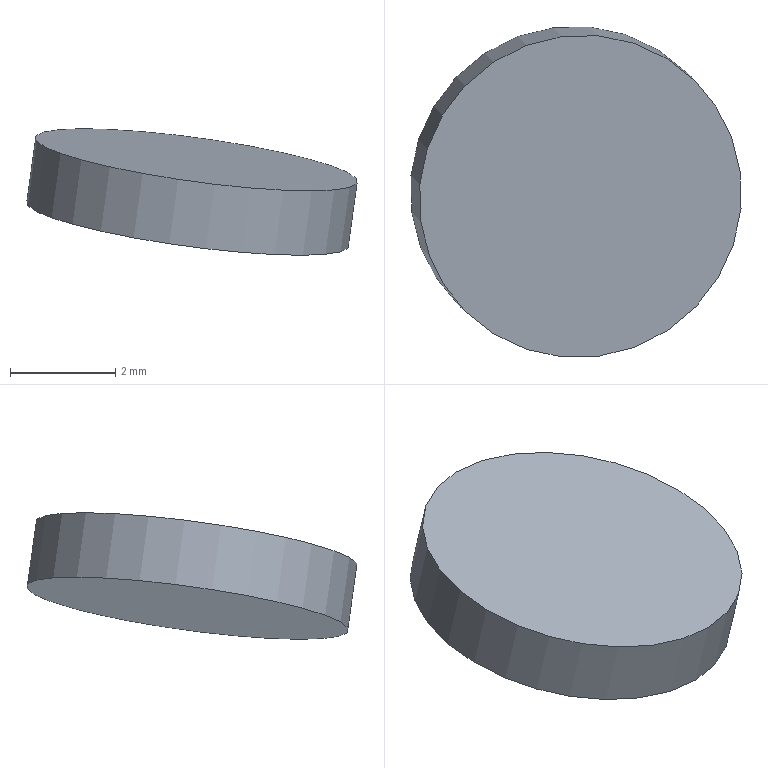Part | STEP file | gslz 2016.10.28-13_id1086_x_t | 1 solid | 3 faces | box 6.311 x 6.312 x 2.41 mm | volume 37.737 mm3 | spline 2 | cylinder 1 | commonest cylinder face diameters 6.2 x1
STEP:
#1=CARTESIAN_POINT('',(0.,0.,0.));
#2=DIRECTION('',(0.,0.,1.));
#3=DIRECTION('',(1.,0.,0.));
#4=AXIS2_PLACEMENT_3D('',#1,#2,#3);
#5=CARTESIAN_POINT('',(775.863,213.366,0.09839));
#6=VERTEX_POINT('',#5);
#7=CARTESIAN_POINT('',(771.479,208.982,0.09841));
#8=VERTEX_POINT('',#7);
#9=CARTESIAN_POINT('',(775.863,213.366,0.09839));
#10=CARTESIAN_POINT('',(775.855,213.374,0.1005));
#11=CARTESIAN_POINT('',(775.848,213.381,0.1026));
#12=CARTESIAN_POINT('',(775.84,213.389,0.1048));
#13=CARTESIAN_POINT('',(775.596,213.627,0.171));
#14=CARTESIAN_POINT('',(775.308,213.826,0.238));
#15=CARTESIAN_POINT('',(774.998,213.969,0.3002));
#16=CARTESIAN_POINT('',(774.688,214.111,0.3624));
#17=CARTESIAN_POINT('',(774.348,214.202,0.4216));
#18=CARTESIAN_POINT('',(774.006,214.233,0.4729));
#19=CARTESIAN_POINT('',(773.664,214.264,0.5241));
#20=CARTESIAN_POINT('',(773.311,214.237,0.5688));
#21=CARTESIAN_POINT('',(772.976,214.153,0.6033));
#22=CARTESIAN_POINT('',(772.641,214.069,0.6378));
#23=CARTESIAN_POINT('',(772.315,213.926,0.663));
#24=CARTESIAN_POINT('',(772.025,213.736,0.6768));
#25=CARTESIAN_POINT('',(771.843,213.618,0.6855));
#26=CARTESIAN_POINT('',(771.673,213.479,0.6899));
#27=CARTESIAN_POINT('',(771.519,213.326,0.6899));
#28=CARTESIAN_POINT('',(771.274,213.08,0.6899));
#29=CARTESIAN_POINT('',(771.067,212.79,0.6785));
#30=CARTESIAN_POINT('',(770.915,212.479,0.6566));
#31=CARTESIAN_POINT('',(770.763,212.168,0.6347));
#32=CARTESIAN_POINT('',(770.663,211.827,0.6017));
#33=CARTESIAN_POINT('',(770.622,211.485,0.5603));
#34=CARTESIAN_POINT('',(770.58,211.143,0.5189));
#35=CARTESIAN_POINT('',(770.598,210.79,0.4681));
#36=CARTESIAN_POINT('',(770.672,210.456,0.412));
#37=CARTESIAN_POINT('',(770.746,210.122,0.3558));
#38=CARTESIAN_POINT('',(770.879,209.797,0.2928));
#39=CARTESIAN_POINT('',(771.06,209.508,0.2283));
#40=CARTESIAN_POINT('',(771.179,209.318,0.1858));
#41=CARTESIAN_POINT('',(771.321,209.14,0.142));
#42=CARTESIAN_POINT('',(771.479,208.982,0.09841));
#43=B_SPLINE_CURVE_WITH_KNOTS('',3,(#9,#10,#11,#12,#13,#14,#15,#16,#17,#18,#19,#20,#21,#22,#23,#24,#25,#26,#27,#28,#29,#30,#31,#32,#33,#34,#35,#36,#37,#38,#39,#40,#41,#42),.UNSPECIFIED.,.F.,.F.,(4,3,3,3,3,3,3,3,3,3,3,4),(0.,0.003402,0.1108,0.2183,0.3257,0.4331,0.4998,0.6072,0.7146,0.822,0.9295,1.),.UNSPECIFIED.);
#44=CARTESIAN_POINT('',(773.503,211.343,-1.129));
#45=DIRECTION('',(0.1349,-0.1349,0.9816));
#46=DIRECTION('',(-0.01175,-0.9908,-0.1346));
#47=AXIS2_PLACEMENT_3D('',#44,#45,#46);
#48=CYLINDRICAL_SURFACE('',#47,3.1);
#49=CARTESIAN_POINT('',(8.642,1.25));
#50=CARTESIAN_POINT('',(11.784,1.25));
#51=B_SPLINE_CURVE_WITH_KNOTS('',1,(#49,#50),.UNSPECIFIED.,.F.,.F.,(2,2),(0.,1.),.PIECEWISE_BEZIER_KNOTS.);
#52=(GEOMETRIC_REPRESENTATION_CONTEXT(2)PARAMETRIC_REPRESENTATION_CONTEXT()REPRESENTATION_CONTEXT('',''));
#53=DEFINITIONAL_REPRESENTATION('',(#51),#52);
#54=PCURVE('',#48,#53);
#55=CARTESIAN_POINT('',(582.842,140.622,16.631));
#56=CARTESIAN_POINT('',(603.987,119.477,10.818));
#57=CARTESIAN_POINT('',(625.133,98.331,5.005));
#58=CARTESIAN_POINT('',(646.279,77.185,-0.8076));
#59=CARTESIAN_POINT('',(667.424,56.039,-6.62));
#60=CARTESIAN_POINT('',(688.57,34.894,-12.433));
#61=CARTESIAN_POINT('',(618.357,176.138,16.631));
#62=CARTESIAN_POINT('',(639.503,154.992,10.818));
#63=CARTESIAN_POINT('',(660.649,133.847,5.005));
#64=CARTESIAN_POINT('',(681.795,112.701,-0.8078));
#65=CARTESIAN_POINT('',(702.94,91.555,-6.621));
#66=CARTESIAN_POINT('',(724.086,70.41,-12.434));
#67=CARTESIAN_POINT('',(653.873,211.654,16.631));
#68=CARTESIAN_POINT('',(675.019,190.508,10.818));
#69=CARTESIAN_POINT('',(696.165,169.363,5.005));
#70=CARTESIAN_POINT('',(717.31,148.217,-0.808));
#71=CARTESIAN_POINT('',(738.456,127.071,-6.621));
#72=CARTESIAN_POINT('',(759.602,105.925,-12.434));
#73=CARTESIAN_POINT('',(689.389,247.17,16.63));
#74=CARTESIAN_POINT('',(710.535,226.024,10.818));
#75=CARTESIAN_POINT('',(731.68,204.878,5.005));
#76=CARTESIAN_POINT('',(752.826,183.733,-0.8082));
#77=CARTESIAN_POINT('',(773.972,162.587,-6.621));
#78=CARTESIAN_POINT('',(795.118,141.441,-12.434));
#79=CARTESIAN_POINT('',(724.905,282.686,16.63));
#80=CARTESIAN_POINT('',(746.051,261.54,10.817));
#81=CARTESIAN_POINT('',(767.196,240.394,5.005));
#82=CARTESIAN_POINT('',(788.342,219.248,-0.8083));
#83=CARTESIAN_POINT('',(809.488,198.103,-6.621));
#84=CARTESIAN_POINT('',(830.633,176.957,-12.434));
#85=CARTESIAN_POINT('',(760.421,318.201,16.63));
#86=CARTESIAN_POINT('',(781.566,297.056,10.817));
#87=CARTESIAN_POINT('',(802.712,275.91,5.004));
#88=CARTESIAN_POINT('',(823.858,254.764,-0.8085));
#89=CARTESIAN_POINT('',(845.003,233.618,-6.621));
#90=CARTESIAN_POINT('',(866.149,212.473,-12.434));
#91=B_SPLINE_SURFACE_WITH_KNOTS('',5,5,((#55,#56,#57,#58,#59,#60),(#61,#62,#63,#64,#65,#66),(#67,#68,#69,#70,#71,#72),(#73,#74,#75,#76,#77,#78),(#79,#80,#81,#82,#83,#84),(#85,#86,#87,#88,#89,#90)),.UNSPECIFIED.,.F.,.F.,.F.,(6,6),(6,6),(0.,1.),(0.,1.),.PIECEWISE_BEZIER_KNOTS.);
#92=CARTESIAN_POINT('',(0.7483,0.5688));
#93=CARTESIAN_POINT('',(0.7483,0.5683));
#94=CARTESIAN_POINT('',(0.7483,0.5674));
#95=CARTESIAN_POINT('',(0.7482,0.5659));
#96=CARTESIAN_POINT('',(0.748,0.5645));
#97=CARTESIAN_POINT('',(0.7478,0.5631));
#98=CARTESIAN_POINT('',(0.7475,0.5617));
#99=CARTESIAN_POINT('',(0.7472,0.5603));
#100=CARTESIAN_POINT('',(0.7468,0.559));
#101=CARTESIAN_POINT('',(0.7463,0.5578));
#102=CARTESIAN_POINT('',(0.7458,0.5566));
#103=CARTESIAN_POINT('',(0.7453,0.5555));
#104=CARTESIAN_POINT('',(0.7447,0.5544));
#105=CARTESIAN_POINT('',(0.744,0.5534));
#106=CARTESIAN_POINT('',(0.7434,0.5525));
#107=CARTESIAN_POINT('',(0.7426,0.5517));
#108=CARTESIAN_POINT('',(0.7419,0.5509));
#109=CARTESIAN_POINT('',(0.7411,0.5503));
#110=CARTESIAN_POINT('',(0.7403,0.5497));
#111=CARTESIAN_POINT('',(0.7394,0.5493));
#112=CARTESIAN_POINT('',(0.7386,0.5489));
#113=CARTESIAN_POINT('',(0.7377,0.5486));
#114=CARTESIAN_POINT('',(0.7368,0.5485));
#115=CARTESIAN_POINT('',(0.7359,0.5484));
#116=CARTESIAN_POINT('',(0.7351,0.5485));
#117=CARTESIAN_POINT('',(0.7342,0.5486));
#118=CARTESIAN_POINT('',(0.7333,0.5489));
#119=CARTESIAN_POINT('',(0.7325,0.5493));
#120=CARTESIAN_POINT('',(0.7316,0.5497));
#121=CARTESIAN_POINT('',(0.7308,0.5503));
#122=CARTESIAN_POINT('',(0.73,0.5509));
#123=CARTESIAN_POINT('',(0.7293,0.5517));
#124=CARTESIAN_POINT('',(0.7285,0.5525));
#125=CARTESIAN_POINT('',(0.7279,0.5534));
#126=CARTESIAN_POINT('',(0.7272,0.5544));
#127=CARTESIAN_POINT('',(0.7266,0.5555));
#128=CARTESIAN_POINT('',(0.7261,0.5566));
#129=CARTESIAN_POINT('',(0.7256,0.5578));
#130=CARTESIAN_POINT('',(0.7251,0.559));
#131=CARTESIAN_POINT('',(0.7247,0.5603));
#132=CARTESIAN_POINT('',(0.7244,0.5617));
#133=CARTESIAN_POINT('',(0.7241,0.5631));
#134=CARTESIAN_POINT('',(0.7239,0.5645));
#135=CARTESIAN_POINT('',(0.7237,0.5659));
#136=CARTESIAN_POINT('',(0.7236,0.5674));
#137=CARTESIAN_POINT('',(0.7236,0.5683));
#138=CARTESIAN_POINT('',(0.7236,0.5688));
#139=B_SPLINE_CURVE_WITH_KNOTS('',3,(#92,#93,#94,#95,#96,#97,#98,#99,#100,#101,#102,#103,#104,#105,#106,#107,#108,#109,#110,#111,#112,#113,#114,#115,#116,#117,#118,#119,#120,#121,#122,#123,#124,#125,#126,#127,#128,#129,#130,#131,#132,#133,#134,#135,#136,#137,#138),.UNSPECIFIED.,.F.,.F.,(4,1,1,1,1,1,1,1,1,1,1,1,1,1,1,1,1,1,1,1,1,1,1,1,1,1,1,1,1,1,1,1,1,1,1,1,1,1,1,1,1,1,1,1,4),(0.,0.02273,0.04545,0.06818,0.09091,0.1136,0.1364,0.1591,0.1818,0.2045,0.2273,0.25,0.2727,0.2955,0.3182,0.3409,0.3636,0.3864,0.4091,0.4318,0.4545,0.4773,0.5,0.5227,0.5455,0.5682,0.5909,0.6136,0.6364,0.6591,0.6818,0.7045,0.7273,0.75,0.7727,0.7955,0.8182,0.8409,0.8636,0.8864,0.9091,0.9318,0.9545,0.9773,1.),.QUASI_UNIFORM_KNOTS.);
#140=(GEOMETRIC_REPRESENTATION_CONTEXT(2)PARAMETRIC_REPRESENTATION_CONTEXT()REPRESENTATION_CONTEXT('',''));
#141=DEFINITIONAL_REPRESENTATION('',(#139),#140);
#142=PCURVE('',#91,#141);
#143=SURFACE_CURVE('',#43,(#54,#142),.PCURVE_S1.);
#144=EDGE_CURVE('',#6,#8,#143,.T.);
#145=ORIENTED_EDGE('',*,*,#144,.F.);
#146=CARTESIAN_POINT('',(771.479,208.982,0.09841));
#147=CARTESIAN_POINT('',(771.487,208.974,0.09629));
#148=CARTESIAN_POINT('',(771.495,208.967,0.09416));
#149=CARTESIAN_POINT('',(771.502,208.959,0.09204));
#150=CARTESIAN_POINT('',(771.746,208.721,0.02584));
#151=CARTESIAN_POINT('',(772.035,208.522,-0.04115));
#152=CARTESIAN_POINT('',(772.345,208.379,-0.1034));
#153=CARTESIAN_POINT('',(772.655,208.237,-0.1656));
#154=CARTESIAN_POINT('',(772.995,208.146,-0.2248));
#155=CARTESIAN_POINT('',(773.337,208.115,-0.2761));
#156=CARTESIAN_POINT('',(773.678,208.084,-0.3273));
#157=CARTESIAN_POINT('',(774.031,208.111,-0.372));
#158=CARTESIAN_POINT('',(774.366,208.195,-0.4065));
#159=CARTESIAN_POINT('',(774.701,208.279,-0.441));
#160=CARTESIAN_POINT('',(775.027,208.422,-0.4662));
#161=CARTESIAN_POINT('',(775.317,208.612,-0.48));
#162=CARTESIAN_POINT('',(775.499,208.73,-0.4887));
#163=CARTESIAN_POINT('',(775.669,208.869,-0.4931));
#164=CARTESIAN_POINT('',(775.823,209.022,-0.4931));
#165=CARTESIAN_POINT('',(776.068,209.268,-0.4931));
#166=CARTESIAN_POINT('',(776.275,209.558,-0.4817));
#167=CARTESIAN_POINT('',(776.427,209.869,-0.4598));
#168=CARTESIAN_POINT('',(776.579,210.18,-0.4379));
#169=CARTESIAN_POINT('',(776.68,210.521,-0.4049));
#170=CARTESIAN_POINT('',(776.721,210.863,-0.3635));
#171=CARTESIAN_POINT('',(776.762,211.205,-0.3221));
#172=CARTESIAN_POINT('',(776.745,211.558,-0.2713));
#173=CARTESIAN_POINT('',(776.67,211.892,-0.2152));
#174=CARTESIAN_POINT('',(776.596,212.226,-0.159));
#175=CARTESIAN_POINT('',(776.463,212.551,-0.09604));
#176=CARTESIAN_POINT('',(776.282,212.84,-0.03145));
#177=CARTESIAN_POINT('',(776.163,213.03,0.01103));
#178=CARTESIAN_POINT('',(776.022,213.208,0.05484));
#179=CARTESIAN_POINT('',(775.863,213.366,0.09839));
#180=B_SPLINE_CURVE_WITH_KNOTS('',3,(#146,#147,#148,#149,#150,#151,#152,#153,#154,#155,#156,#157,#158,#159,#160,#161,#162,#163,#164,#165,#166,#167,#168,#169,#170,#171,#172,#173,#174,#175,#176,#177,#178,#179),.UNSPECIFIED.,.F.,.F.,(4,3,3,3,3,3,3,3,3,3,3,4),(0.,0.003402,0.1108,0.2183,0.3257,0.4331,0.4998,0.6072,0.7146,0.822,0.9295,1.),.UNSPECIFIED.);
#181=CARTESIAN_POINT('',(5.5,1.25));
#182=CARTESIAN_POINT('',(8.642,1.25));
#183=B_SPLINE_CURVE_WITH_KNOTS('',1,(#181,#182),.UNSPECIFIED.,.F.,.F.,(2,2),(0.,1.),.PIECEWISE_BEZIER_KNOTS.);
#184=(GEOMETRIC_REPRESENTATION_CONTEXT(2)PARAMETRIC_REPRESENTATION_CONTEXT()REPRESENTATION_CONTEXT('',''));
#185=DEFINITIONAL_REPRESENTATION('',(#183),#184);
#186=PCURVE('',#48,#185);
#187=CARTESIAN_POINT('',(0.7236,0.5688));
#188=CARTESIAN_POINT('',(0.7236,0.5693));
#189=CARTESIAN_POINT('',(0.7236,0.5703));
#190=CARTESIAN_POINT('',(0.7237,0.5717));
#191=CARTESIAN_POINT('',(0.7239,0.5731));
#192=CARTESIAN_POINT('',(0.7241,0.5745));
#193=CARTESIAN_POINT('',(0.7244,0.5759));
#194=CARTESIAN_POINT('',(0.7247,0.5773));
#195=CARTESIAN_POINT('',(0.7251,0.5786));
#196=CARTESIAN_POINT('',(0.7256,0.5798));
#197=CARTESIAN_POINT('',(0.7261,0.581));
#198=CARTESIAN_POINT('',(0.7266,0.5821));
#199=CARTESIAN_POINT('',(0.7272,0.5832));
#200=CARTESIAN_POINT('',(0.7279,0.5842));
#201=CARTESIAN_POINT('',(0.7286,0.5851));
#202=CARTESIAN_POINT('',(0.7293,0.5859));
#203=CARTESIAN_POINT('',(0.73,0.5867));
#204=CARTESIAN_POINT('',(0.7308,0.5873));
#205=CARTESIAN_POINT('',(0.7316,0.5879));
#206=CARTESIAN_POINT('',(0.7325,0.5883));
#207=CARTESIAN_POINT('',(0.7333,0.5887));
#208=CARTESIAN_POINT('',(0.7342,0.589));
#209=CARTESIAN_POINT('',(0.7351,0.5891));
#210=CARTESIAN_POINT('',(0.736,0.5892));
#211=CARTESIAN_POINT('',(0.7368,0.5891));
#212=CARTESIAN_POINT('',(0.7377,0.589));
#213=CARTESIAN_POINT('',(0.7386,0.5887));
#214=CARTESIAN_POINT('',(0.7394,0.5883));
#215=CARTESIAN_POINT('',(0.7403,0.5879));
#216=CARTESIAN_POINT('',(0.7411,0.5873));
#217=CARTESIAN_POINT('',(0.7419,0.5867));
#218=CARTESIAN_POINT('',(0.7426,0.5859));
#219=CARTESIAN_POINT('',(0.7434,0.5851));
#220=CARTESIAN_POINT('',(0.7441,0.5842));
#221=CARTESIAN_POINT('',(0.7447,0.5832));
#222=CARTESIAN_POINT('',(0.7453,0.5821));
#223=CARTESIAN_POINT('',(0.7459,0.581));
#224=CARTESIAN_POINT('',(0.7464,0.5798));
#225=CARTESIAN_POINT('',(0.7468,0.5786));
#226=CARTESIAN_POINT('',(0.7472,0.5773));
#227=CARTESIAN_POINT('',(0.7475,0.5759));
#228=CARTESIAN_POINT('',(0.7478,0.5745));
#229=CARTESIAN_POINT('',(0.748,0.5731));
#230=CARTESIAN_POINT('',(0.7482,0.5717));
#231=CARTESIAN_POINT('',(0.7483,0.5703));
#232=CARTESIAN_POINT('',(0.7483,0.5693));
#233=CARTESIAN_POINT('',(0.7483,0.5688));
#234=B_SPLINE_CURVE_WITH_KNOTS('',3,(#187,#188,#189,#190,#191,#192,#193,#194,#195,#196,#197,#198,#199,#200,#201,#202,#203,#204,#205,#206,#207,#208,#209,#210,#211,#212,#213,#214,#215,#216,#217,#218,#219,#220,#221,#222,#223,#224,#225,#226,#227,#228,#229,#230,#231,#232,#233),.UNSPECIFIED.,.F.,.F.,(4,1,1,1,1,1,1,1,1,1,1,1,1,1,1,1,1,1,1,1,1,1,1,1,1,1,1,1,1,1,1,1,1,1,1,1,1,1,1,1,1,1,1,1,4),(0.,0.02273,0.04545,0.06818,0.09091,0.1136,0.1364,0.1591,0.1818,0.2045,0.2273,0.25,0.2727,0.2955,0.3182,0.3409,0.3636,0.3864,0.4091,0.4318,0.4545,0.4773,0.5,0.5227,0.5455,0.5682,0.5909,0.6136,0.6364,0.6591,0.6818,0.7045,0.7273,0.75,0.7727,0.7955,0.8182,0.8409,0.8636,0.8864,0.9091,0.9318,0.9545,0.9773,1.),.QUASI_UNIFORM_KNOTS.);
#235=(GEOMETRIC_REPRESENTATION_CONTEXT(2)PARAMETRIC_REPRESENTATION_CONTEXT()REPRESENTATION_CONTEXT('',''));
#236=DEFINITIONAL_REPRESENTATION('',(#234),#235);
#237=PCURVE('',#91,#236);
#238=SURFACE_CURVE('',#180,(#186,#237),.PCURVE_S1.);
#239=EDGE_CURVE('',#8,#6,#238,.T.);
#240=ORIENTED_EDGE('',*,*,#239,.F.);
#241=CARTESIAN_POINT('',(771.31,209.151,-1.129));
#242=VERTEX_POINT('',#241);
#243=CARTESIAN_POINT('',(771.31,209.151,-1.129));
#244=CARTESIAN_POINT('',(771.479,208.982,0.09841));
#245=B_SPLINE_CURVE_WITH_KNOTS('',1,(#243,#244),.UNSPECIFIED.,.F.,.F.,(2,2),(0.,1.25),.PIECEWISE_BEZIER_KNOTS.);
#246=CARTESIAN_POINT('',(5.5,0.));
#247=DIRECTION('',(0.,1.));
#248=VECTOR('',#247,1.);
#249=LINE('',#246,#248);
#250=(GEOMETRIC_REPRESENTATION_CONTEXT(2)PARAMETRIC_REPRESENTATION_CONTEXT()REPRESENTATION_CONTEXT('',''));
#251=DEFINITIONAL_REPRESENTATION('',(#249),#250);
#252=PCURVE('',#48,#251);
#253=CARTESIAN_POINT('',(11.784,0.));
#254=DIRECTION('',(0.,1.));
#255=VECTOR('',#254,1.);
#256=LINE('',#253,#255);
#257=(GEOMETRIC_REPRESENTATION_CONTEXT(2)PARAMETRIC_REPRESENTATION_CONTEXT()REPRESENTATION_CONTEXT('',''));
#258=DEFINITIONAL_REPRESENTATION('',(#256),#257);
#259=PCURVE('',#48,#258);
#260=SEAM_CURVE('',#245,(#252,#259),.PCURVE_S1.);
#261=EDGE_CURVE('',#242,#8,#260,.T.);
#262=ORIENTED_EDGE('',*,*,#261,.F.);
#263=CARTESIAN_POINT('',(775.695,213.535,-1.129));
#264=VERTEX_POINT('',#263);
#265=CARTESIAN_POINT('',(771.31,209.151,-1.129));
#266=CARTESIAN_POINT('',(771.318,209.143,-1.131));
#267=CARTESIAN_POINT('',(771.326,209.135,-1.133));
#268=CARTESIAN_POINT('',(771.334,209.128,-1.135));
#269=CARTESIAN_POINT('',(771.577,208.889,-1.201));
#270=CARTESIAN_POINT('',(771.866,208.691,-1.268));
#271=CARTESIAN_POINT('',(772.176,208.548,-1.33));
#272=CARTESIAN_POINT('',(772.486,208.405,-1.393));
#273=CARTESIAN_POINT('',(772.826,208.315,-1.452));
#274=CARTESIAN_POINT('',(773.168,208.284,-1.503));
#275=CARTESIAN_POINT('',(773.51,208.253,-1.554));
#276=CARTESIAN_POINT('',(773.863,208.28,-1.599));
#277=CARTESIAN_POINT('',(774.197,208.364,-1.634));
#278=CARTESIAN_POINT('',(774.532,208.448,-1.668));
#279=CARTESIAN_POINT('',(774.858,208.591,-1.693));
#280=CARTESIAN_POINT('',(775.149,208.78,-1.707));
#281=CARTESIAN_POINT('',(775.33,208.899,-1.716));
#282=CARTESIAN_POINT('',(775.501,209.037,-1.72));
#283=CARTESIAN_POINT('',(775.654,209.191,-1.72));
#284=CARTESIAN_POINT('',(775.9,209.436,-1.72));
#285=CARTESIAN_POINT('',(776.107,209.727,-1.709));
#286=CARTESIAN_POINT('',(776.259,210.038,-1.687));
#287=CARTESIAN_POINT('',(776.41,210.349,-1.665));
#288=CARTESIAN_POINT('',(776.511,210.69,-1.632));
#289=CARTESIAN_POINT('',(776.552,211.032,-1.591));
#290=CARTESIAN_POINT('',(776.593,211.374,-1.549));
#291=CARTESIAN_POINT('',(776.576,211.727,-1.498));
#292=CARTESIAN_POINT('',(776.502,212.061,-1.442));
#293=CARTESIAN_POINT('',(776.428,212.395,-1.386));
#294=CARTESIAN_POINT('',(776.295,212.72,-1.323));
#295=CARTESIAN_POINT('',(776.113,213.009,-1.258));
#296=CARTESIAN_POINT('',(775.994,213.199,-1.216));
#297=CARTESIAN_POINT('',(775.853,213.376,-1.172));
#298=CARTESIAN_POINT('',(775.695,213.535,-1.129));
#299=B_SPLINE_CURVE_WITH_KNOTS('',3,(#265,#266,#267,#268,#269,#270,#271,#272,#273,#274,#275,#276,#277,#278,#279,#280,#281,#282,#283,#284,#285,#286,#287,#288,#289,#290,#291,#292,#293,#294,#295,#296,#297,#298),.UNSPECIFIED.,.F.,.F.,(4,3,3,3,3,3,3,3,3,3,3,4),(0.,0.003402,0.1108,0.2183,0.3257,0.4331,0.4998,0.6072,0.7146,0.822,0.9295,1.),.UNSPECIFIED.);
#300=CARTESIAN_POINT('',(5.5,0.));
#301=CARTESIAN_POINT('',(8.642,0.));
#302=B_SPLINE_CURVE_WITH_KNOTS('',1,(#300,#301),.UNSPECIFIED.,.F.,.F.,(2,2),(0.,1.),.PIECEWISE_BEZIER_KNOTS.);
#303=(GEOMETRIC_REPRESENTATION_CONTEXT(2)PARAMETRIC_REPRESENTATION_CONTEXT()REPRESENTATION_CONTEXT('',''));
#304=DEFINITIONAL_REPRESENTATION('',(#302),#303);
#305=PCURVE('',#48,#304);
#306=CARTESIAN_POINT('',(769.107,211.302,-0.53));
#307=CARTESIAN_POINT('',(770.558,209.85,-0.9291));
#308=CARTESIAN_POINT('',(772.01,208.399,-1.328));
#309=CARTESIAN_POINT('',(773.462,206.947,-1.727));
#310=CARTESIAN_POINT('',(770.585,212.781,-0.53));
#311=CARTESIAN_POINT('',(772.037,211.329,-0.9291));
#312=CARTESIAN_POINT('',(773.489,209.877,-1.328));
#313=CARTESIAN_POINT('',(774.941,208.426,-1.727));
#314=CARTESIAN_POINT('',(772.064,214.26,-0.53));
#315=CARTESIAN_POINT('',(773.516,212.808,-0.9291));
#316=CARTESIAN_POINT('',(774.968,211.356,-1.328));
#317=CARTESIAN_POINT('',(776.42,209.905,-1.727));
#318=CARTESIAN_POINT('',(773.543,215.739,-0.53));
#319=CARTESIAN_POINT('',(774.995,214.287,-0.9291));
#320=CARTESIAN_POINT('',(776.447,212.835,-1.328));
#321=CARTESIAN_POINT('',(777.898,211.383,-1.727));
#322=B_SPLINE_SURFACE_WITH_KNOTS('',3,3,((#306,#307,#308,#309),(#310,#311,#312,#313),(#314,#315,#316,#317),(#318,#319,#320,#321)),.UNSPECIFIED.,.F.,.F.,.F.,(4,4),(4,4),(0.,1.),(0.,1.),.PIECEWISE_BEZIER_KNOTS.);
#323=CARTESIAN_POINT('',(0.005929,0.5));
#324=CARTESIAN_POINT('',(0.005927,0.5117));
#325=CARTESIAN_POINT('',(0.006781,0.5352));
#326=CARTESIAN_POINT('',(0.01059,0.5703));
#327=CARTESIAN_POINT('',(0.01687,0.6052));
#328=CARTESIAN_POINT('',(0.02559,0.6394));
#329=CARTESIAN_POINT('',(0.03666,0.6728));
#330=CARTESIAN_POINT('',(0.05017,0.7053));
#331=CARTESIAN_POINT('',(0.06601,0.7369));
#332=CARTESIAN_POINT('',(0.08405,0.7673));
#333=CARTESIAN_POINT('',(0.1042,0.7964));
#334=CARTESIAN_POINT('',(0.1262,0.8237));
#335=CARTESIAN_POINT('',(0.1502,0.8495));
#336=CARTESIAN_POINT('',(0.1761,0.8736));
#337=CARTESIAN_POINT('',(0.2037,0.8958));
#338=CARTESIAN_POINT('',(0.2326,0.916));
#339=CARTESIAN_POINT('',(0.2628,0.9339));
#340=CARTESIAN_POINT('',(0.2944,0.9497));
#341=CARTESIAN_POINT('',(0.3271,0.9632));
#342=CARTESIAN_POINT('',(0.3606,0.9744));
#343=CARTESIAN_POINT('',(0.3946,0.9831));
#344=CARTESIAN_POINT('',(0.4296,0.9895));
#345=CARTESIAN_POINT('',(0.4649,0.9932));
#346=CARTESIAN_POINT('',(0.5005,0.9945));
#347=CARTESIAN_POINT('',(0.5355,0.9932));
#348=CARTESIAN_POINT('',(0.5707,0.9894));
#349=CARTESIAN_POINT('',(0.6055,0.9831));
#350=CARTESIAN_POINT('',(0.6397,0.9743));
#351=CARTESIAN_POINT('',(0.673,0.9632));
#352=CARTESIAN_POINT('',(0.7056,0.9497));
#353=CARTESIAN_POINT('',(0.7372,0.9338));
#354=CARTESIAN_POINT('',(0.7676,0.9158));
#355=CARTESIAN_POINT('',(0.7966,0.8956));
#356=CARTESIAN_POINT('',(0.8239,0.8736));
#357=CARTESIAN_POINT('',(0.8498,0.8495));
#358=CARTESIAN_POINT('',(0.8738,0.8236));
#359=CARTESIAN_POINT('',(0.896,0.7961));
#360=CARTESIAN_POINT('',(0.9161,0.7671));
#361=CARTESIAN_POINT('',(0.934,0.7369));
#362=CARTESIAN_POINT('',(0.9498,0.7053));
#363=CARTESIAN_POINT('',(0.9633,0.6726));
#364=CARTESIAN_POINT('',(0.9745,0.639));
#365=CARTESIAN_POINT('',(0.9832,0.605));
#366=CARTESIAN_POINT('',(0.9895,0.5703));
#367=CARTESIAN_POINT('',(0.9932,0.5352));
#368=CARTESIAN_POINT('',(0.9941,0.5117));
#369=CARTESIAN_POINT('',(0.9941,0.5));
#370=B_SPLINE_CURVE_WITH_KNOTS('',3,(#323,#324,#325,#326,#327,#328,#329,#330,#331,#332,#333,#334,#335,#336,#337,#338,#339,#340,#341,#342,#343,#344,#345,#346,#347,#348,#349,#350,#351,#352,#353,#354,#355,#356,#357,#358,#359,#360,#361,#362,#363,#364,#365,#366,#367,#368,#369),.UNSPECIFIED.,.F.,.F.,(4,1,1,1,1,1,1,1,1,1,1,1,1,1,1,1,1,1,1,1,1,1,1,1,1,1,1,1,1,1,1,1,1,1,1,1,1,1,1,1,1,1,1,1,4),(0.,0.02273,0.04545,0.06818,0.09091,0.1136,0.1364,0.1591,0.1818,0.2045,0.2273,0.25,0.2727,0.2955,0.3182,0.3409,0.3636,0.3864,0.4091,0.4318,0.4545,0.4773,0.5,0.5227,0.5455,0.5682,0.5909,0.6136,0.6364,0.6591,0.6818,0.7045,0.7273,0.75,0.7727,0.7955,0.8182,0.8409,0.8636,0.8864,0.9091,0.9318,0.9545,0.9773,1.),.QUASI_UNIFORM_KNOTS.);
#371=(GEOMETRIC_REPRESENTATION_CONTEXT(2)PARAMETRIC_REPRESENTATION_CONTEXT()REPRESENTATION_CONTEXT('',''));
#372=DEFINITIONAL_REPRESENTATION('',(#370),#371);
#373=PCURVE('',#322,#372);
#374=SURFACE_CURVE('',#299,(#305,#373),.PCURVE_S1.);
#375=EDGE_CURVE('',#242,#264,#374,.T.);
#376=ORIENTED_EDGE('',*,*,#375,.T.);
#377=CARTESIAN_POINT('',(775.695,213.535,-1.129));
#378=CARTESIAN_POINT('',(775.687,213.542,-1.127));
#379=CARTESIAN_POINT('',(775.679,213.55,-1.124));
#380=CARTESIAN_POINT('',(775.671,213.558,-1.122));
#381=CARTESIAN_POINT('',(775.428,213.796,-1.056));
#382=CARTESIAN_POINT('',(775.139,213.995,-0.9891));
#383=CARTESIAN_POINT('',(774.829,214.137,-0.9268));
#384=CARTESIAN_POINT('',(774.519,214.28,-0.8646));
#385=CARTESIAN_POINT('',(774.179,214.371,-0.8054));
#386=CARTESIAN_POINT('',(773.837,214.402,-0.7542));
#387=CARTESIAN_POINT('',(773.495,214.433,-0.7029));
#388=CARTESIAN_POINT('',(773.142,214.405,-0.6582));
#389=CARTESIAN_POINT('',(772.808,214.321,-0.6237));
#390=CARTESIAN_POINT('',(772.473,214.237,-0.5892));
#391=CARTESIAN_POINT('',(772.147,214.095,-0.564));
#392=CARTESIAN_POINT('',(771.856,213.905,-0.5502));
#393=CARTESIAN_POINT('',(771.675,213.786,-0.5415));
#394=CARTESIAN_POINT('',(771.504,213.648,-0.5371));
#395=CARTESIAN_POINT('',(771.351,213.494,-0.5371));
#396=CARTESIAN_POINT('',(771.105,213.249,-0.5371));
#397=CARTESIAN_POINT('',(770.898,212.959,-0.5486));
#398=CARTESIAN_POINT('',(770.746,212.648,-0.5705));
#399=CARTESIAN_POINT('',(770.595,212.336,-0.5924));
#400=CARTESIAN_POINT('',(770.494,211.996,-0.6254));
#401=CARTESIAN_POINT('',(770.453,211.654,-0.6667));
#402=CARTESIAN_POINT('',(770.412,211.312,-0.7081));
#403=CARTESIAN_POINT('',(770.429,210.959,-0.7589));
#404=CARTESIAN_POINT('',(770.503,210.625,-0.8151));
#405=CARTESIAN_POINT('',(770.577,210.29,-0.8712));
#406=CARTESIAN_POINT('',(770.71,209.965,-0.9342));
#407=CARTESIAN_POINT('',(770.892,209.676,-0.9988));
#408=CARTESIAN_POINT('',(771.011,209.487,-1.041));
#409=CARTESIAN_POINT('',(771.152,209.309,-1.085));
#410=CARTESIAN_POINT('',(771.31,209.151,-1.129));
#411=B_SPLINE_CURVE_WITH_KNOTS('',3,(#377,#378,#379,#380,#381,#382,#383,#384,#385,#386,#387,#388,#389,#390,#391,#392,#393,#394,#395,#396,#397,#398,#399,#400,#401,#402,#403,#404,#405,#406,#407,#408,#409,#410),.UNSPECIFIED.,.F.,.F.,(4,3,3,3,3,3,3,3,3,3,3,4),(0.,0.003402,0.1108,0.2183,0.3257,0.4331,0.4998,0.6072,0.7146,0.822,0.9295,1.),.UNSPECIFIED.);
#412=CARTESIAN_POINT('',(8.642,0.));
#413=CARTESIAN_POINT('',(11.784,0.));
#414=B_SPLINE_CURVE_WITH_KNOTS('',1,(#412,#413),.UNSPECIFIED.,.F.,.F.,(2,2),(0.,1.),.PIECEWISE_BEZIER_KNOTS.);
#415=(GEOMETRIC_REPRESENTATION_CONTEXT(2)PARAMETRIC_REPRESENTATION_CONTEXT()REPRESENTATION_CONTEXT('',''));
#416=DEFINITIONAL_REPRESENTATION('',(#414),#415);
#417=PCURVE('',#48,#416);
#418=CARTESIAN_POINT('',(0.9941,0.5));
#419=CARTESIAN_POINT('',(0.9941,0.4883));
#420=CARTESIAN_POINT('',(0.9932,0.4648));
#421=CARTESIAN_POINT('',(0.9894,0.4297));
#422=CARTESIAN_POINT('',(0.9831,0.3948));
#423=CARTESIAN_POINT('',(0.9744,0.3606));
#424=CARTESIAN_POINT('',(0.9633,0.3272));
#425=CARTESIAN_POINT('',(0.9498,0.2947));
#426=CARTESIAN_POINT('',(0.934,0.2631));
#427=CARTESIAN_POINT('',(0.9159,0.2327));
#428=CARTESIAN_POINT('',(0.8958,0.2036));
#429=CARTESIAN_POINT('',(0.8738,0.1763));
#430=CARTESIAN_POINT('',(0.8498,0.1505));
#431=CARTESIAN_POINT('',(0.8239,0.1264));
#432=CARTESIAN_POINT('',(0.7963,0.1042));
#433=CARTESIAN_POINT('',(0.7674,0.08404));
#434=CARTESIAN_POINT('',(0.7372,0.06612));
#435=CARTESIAN_POINT('',(0.7056,0.05032));
#436=CARTESIAN_POINT('',(0.6729,0.03678));
#437=CARTESIAN_POINT('',(0.6394,0.02558));
#438=CARTESIAN_POINT('',(0.6054,0.01686));
#439=CARTESIAN_POINT('',(0.5704,0.01055));
#440=CARTESIAN_POINT('',(0.5351,0.006757));
#441=CARTESIAN_POINT('',(0.4995,0.005501));
#442=CARTESIAN_POINT('',(0.4645,0.006811));
#443=CARTESIAN_POINT('',(0.4293,0.01064));
#444=CARTESIAN_POINT('',(0.3945,0.01694));
#445=CARTESIAN_POINT('',(0.3603,0.02567));
#446=CARTESIAN_POINT('',(0.327,0.03677));
#447=CARTESIAN_POINT('',(0.2944,0.05032));
#448=CARTESIAN_POINT('',(0.2628,0.06618));
#449=CARTESIAN_POINT('',(0.2324,0.08424));
#450=CARTESIAN_POINT('',(0.2034,0.1044));
#451=CARTESIAN_POINT('',(0.1761,0.1264));
#452=CARTESIAN_POINT('',(0.1502,0.1505));
#453=CARTESIAN_POINT('',(0.1262,0.1764));
#454=CARTESIAN_POINT('',(0.104,0.2039));
#455=CARTESIAN_POINT('',(0.08387,0.2329));
#456=CARTESIAN_POINT('',(0.06597,0.2631));
#457=CARTESIAN_POINT('',(0.05018,0.2947));
#458=CARTESIAN_POINT('',(0.03666,0.3274));
#459=CARTESIAN_POINT('',(0.02548,0.361));
#460=CARTESIAN_POINT('',(0.01678,0.395));
#461=CARTESIAN_POINT('',(0.01054,0.4297));
#462=CARTESIAN_POINT('',(0.006773,0.4648));
#463=CARTESIAN_POINT('',(0.005929,0.4883));
#464=CARTESIAN_POINT('',(0.005929,0.5));
#465=B_SPLINE_CURVE_WITH_KNOTS('',3,(#418,#419,#420,#421,#422,#423,#424,#425,#426,#427,#428,#429,#430,#431,#432,#433,#434,#435,#436,#437,#438,#439,#440,#441,#442,#443,#444,#445,#446,#447,#448,#449,#450,#451,#452,#453,#454,#455,#456,#457,#458,#459,#460,#461,#462,#463,#464),.UNSPECIFIED.,.F.,.F.,(4,1,1,1,1,1,1,1,1,1,1,1,1,1,1,1,1,1,1,1,1,1,1,1,1,1,1,1,1,1,1,1,1,1,1,1,1,1,1,1,1,1,1,1,4),(0.,0.02273,0.04545,0.06818,0.09091,0.1136,0.1364,0.1591,0.1818,0.2045,0.2273,0.25,0.2727,0.2955,0.3182,0.3409,0.3636,0.3864,0.4091,0.4318,0.4545,0.4773,0.5,0.5227,0.5455,0.5682,0.5909,0.6136,0.6364,0.6591,0.6818,0.7045,0.7273,0.75,0.7727,0.7955,0.8182,0.8409,0.8636,0.8864,0.9091,0.9318,0.9545,0.9773,1.),.QUASI_UNIFORM_KNOTS.);
#466=(GEOMETRIC_REPRESENTATION_CONTEXT(2)PARAMETRIC_REPRESENTATION_CONTEXT()REPRESENTATION_CONTEXT('',''));
#467=DEFINITIONAL_REPRESENTATION('',(#465),#466);
#468=PCURVE('',#322,#467);
#469=SURFACE_CURVE('',#411,(#417,#468),.PCURVE_S1.);
#470=EDGE_CURVE('',#264,#242,#469,.T.);
#471=ORIENTED_EDGE('',*,*,#470,.T.);
#472=ORIENTED_EDGE('',*,*,#261,.T.);
#473=EDGE_LOOP('',(#145,#240,#262,#376,#471,#472));
#474=FACE_BOUND('',#473,.T.);
#475=ADVANCED_FACE('',(#474),#48,.T.);
#476=ORIENTED_EDGE('',*,*,#470,.F.);
#477=ORIENTED_EDGE('',*,*,#375,.F.);
#478=EDGE_LOOP('',(#476,#477));
#479=FACE_BOUND('',#478,.T.);
#480=ADVANCED_FACE('',(#479),#322,.T.);
#481=ORIENTED_EDGE('',*,*,#239,.F.);
#482=ORIENTED_EDGE('',*,*,#144,.F.);
#483=EDGE_LOOP('',(#481,#482));
#484=FACE_BOUND('',#483,.F.);
#485=ADVANCED_FACE('',(#484),#91,.F.);
#486=CLOSED_SHELL('',(#475,#480,#485));
#487=MANIFOLD_SOLID_BREP('',#486);
#488=(LENGTH_UNIT()NAMED_UNIT(*)SI_UNIT(.MILLI.,.METRE.));
#489=UNCERTAINTY_MEASURE_WITH_UNIT(LENGTH_MEASURE(0.002),#488,'','');
#490=(NAMED_UNIT(*)PLANE_ANGLE_UNIT()SI_UNIT($,.RADIAN.));
#491=(NAMED_UNIT(*)SI_UNIT($,.STERADIAN.)SOLID_ANGLE_UNIT());
#492=(GEOMETRIC_REPRESENTATION_CONTEXT(3)GLOBAL_UNCERTAINTY_ASSIGNED_CONTEXT((#489))GLOBAL_UNIT_ASSIGNED_CONTEXT((#488,#490,#491))REPRESENTATION_CONTEXT('',''));
#493=ADVANCED_BREP_SHAPE_REPRESENTATION('',(#4,#487),#492);